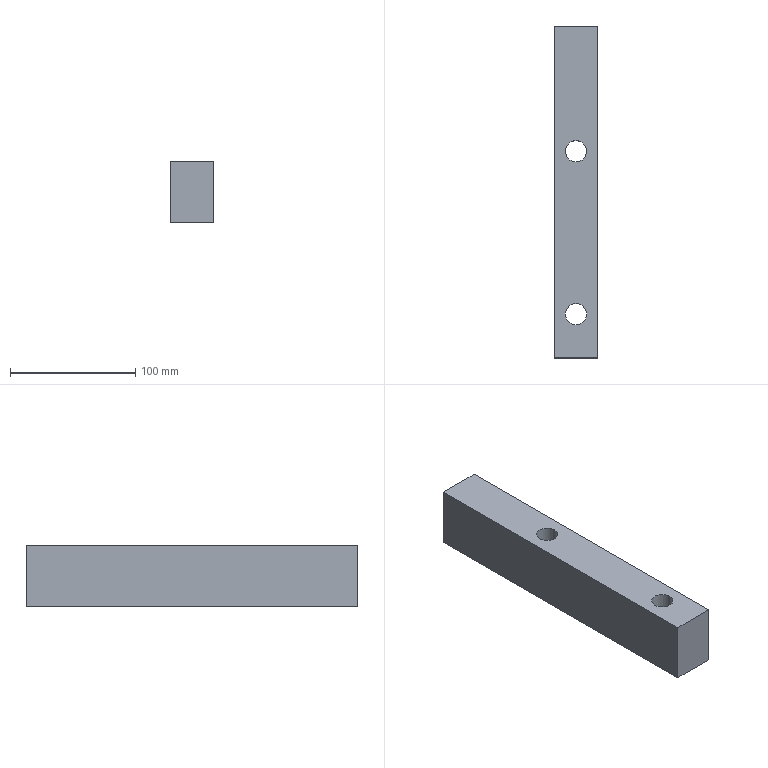Part | NX | features solid 2 | 1 solid | 8 faces | box 35 x 265 x 49 mm | volume 432231 mm3 | plane 6 | cylinder 2 | commonest cylinder face diameters 17 x2
STEP:
#1=CARTESIAN_POINT('',(668.,370.,153.));
#2=VERTEX_POINT('',#1);
#3=CARTESIAN_POINT('',(668.,370.,202.));
#4=VERTEX_POINT('',#3);
#5=CARTESIAN_POINT('',(668.,370.,148.));
#6=DIRECTION('',(0.,0.,1.));
#7=VECTOR('',#6,1000.);
#8=LINE('',#5,#7);
#9=EDGE_CURVE('',#2,#4,#8,.T.);
#10=ORIENTED_EDGE('',*,*,#9,.F.);
#11=CARTESIAN_POINT('',(668.,105.,153.));
#12=VERTEX_POINT('',#11);
#13=CARTESIAN_POINT('',(668.,0.,153.));
#14=DIRECTION('',(0.,-1.,0.));
#15=VECTOR('',#14,1000.);
#16=LINE('',#13,#15);
#17=EDGE_CURVE('',#2,#12,#16,.T.);
#18=ORIENTED_EDGE('',*,*,#17,.T.);
#19=CARTESIAN_POINT('',(668.,105.,202.));
#20=VERTEX_POINT('',#19);
#21=CARTESIAN_POINT('',(668.,105.,148.));
#22=DIRECTION('',(0.,0.,1.));
#23=VECTOR('',#22,1000.);
#24=LINE('',#21,#23);
#25=EDGE_CURVE('',#12,#20,#24,.T.);
#26=ORIENTED_EDGE('',*,*,#25,.T.);
#27=CARTESIAN_POINT('',(668.,0.,202.));
#28=DIRECTION('',(0.,1.,0.));
#29=VECTOR('',#28,1000.);
#30=LINE('',#27,#29);
#31=EDGE_CURVE('',#20,#4,#30,.T.);
#32=ORIENTED_EDGE('',*,*,#31,.T.);
#33=EDGE_LOOP('',(#10,#18,#26,#32));
#34=FACE_BOUND('',#33,.T.);
#35=CARTESIAN_POINT('',(668.,0.,148.));
#36=DIRECTION('',(-1.,0.,0.));
#37=DIRECTION('',(0.,0.,1.));
#38=AXIS2_PLACEMENT_3D('',#35,#36,#37);
#39=PLANE('',#38);
#40=ADVANCED_FACE('',(#34),#39,.T.);
#41=CARTESIAN_POINT('',(703.,370.,153.));
#42=VERTEX_POINT('',#41);
#43=CARTESIAN_POINT('',(703.,370.,202.));
#44=VERTEX_POINT('',#43);
#45=CARTESIAN_POINT('',(703.,370.,148.));
#46=DIRECTION('',(0.,0.,1.));
#47=VECTOR('',#46,1000.);
#48=LINE('',#45,#47);
#49=EDGE_CURVE('',#42,#44,#48,.T.);
#50=ORIENTED_EDGE('',*,*,#49,.F.);
#51=CARTESIAN_POINT('',(685.5,370.,153.));
#52=DIRECTION('',(-1.,0.,0.));
#53=VECTOR('',#52,1000.);
#54=LINE('',#51,#53);
#55=EDGE_CURVE('',#42,#2,#54,.T.);
#56=ORIENTED_EDGE('',*,*,#55,.T.);
#57=ORIENTED_EDGE('',*,*,#9,.T.);
#58=CARTESIAN_POINT('',(685.5,370.,202.));
#59=DIRECTION('',(1.,0.,0.));
#60=VECTOR('',#59,1000.);
#61=LINE('',#58,#60);
#62=EDGE_CURVE('',#4,#44,#61,.T.);
#63=ORIENTED_EDGE('',*,*,#62,.T.);
#64=EDGE_LOOP('',(#50,#56,#57,#63));
#65=FACE_BOUND('',#64,.T.);
#66=CARTESIAN_POINT('',(685.5,370.,148.));
#67=DIRECTION('',(0.,1.,0.));
#68=DIRECTION('',(0.,0.,1.));
#69=AXIS2_PLACEMENT_3D('',#66,#67,#68);
#70=PLANE('',#69);
#71=ADVANCED_FACE('',(#65),#70,.T.);
#72=CARTESIAN_POINT('',(703.,105.,153.));
#73=VERTEX_POINT('',#72);
#74=CARTESIAN_POINT('',(703.,105.,202.));
#75=VERTEX_POINT('',#74);
#76=CARTESIAN_POINT('',(703.,105.,148.));
#77=DIRECTION('',(0.,0.,1.));
#78=VECTOR('',#77,1000.);
#79=LINE('',#76,#78);
#80=EDGE_CURVE('',#73,#75,#79,.T.);
#81=ORIENTED_EDGE('',*,*,#80,.F.);
#82=CARTESIAN_POINT('',(703.,0.,153.));
#83=DIRECTION('',(0.,1.,0.));
#84=VECTOR('',#83,1000.);
#85=LINE('',#82,#84);
#86=EDGE_CURVE('',#73,#42,#85,.T.);
#87=ORIENTED_EDGE('',*,*,#86,.T.);
#88=ORIENTED_EDGE('',*,*,#49,.T.);
#89=CARTESIAN_POINT('',(703.,0.,202.));
#90=DIRECTION('',(0.,-1.,0.));
#91=VECTOR('',#90,1000.);
#92=LINE('',#89,#91);
#93=EDGE_CURVE('',#44,#75,#92,.T.);
#94=ORIENTED_EDGE('',*,*,#93,.T.);
#95=EDGE_LOOP('',(#81,#87,#88,#94));
#96=FACE_BOUND('',#95,.T.);
#97=CARTESIAN_POINT('',(703.,0.,148.));
#98=DIRECTION('',(1.,0.,0.));
#99=DIRECTION('',(0.,0.,-1.));
#100=AXIS2_PLACEMENT_3D('',#97,#98,#99);
#101=PLANE('',#100);
#102=ADVANCED_FACE('',(#96),#101,.T.);
#103=ORIENTED_EDGE('',*,*,#25,.F.);
#104=CARTESIAN_POINT('',(685.5,105.,153.));
#105=DIRECTION('',(1.,0.,0.));
#106=VECTOR('',#105,1000.);
#107=LINE('',#104,#106);
#108=EDGE_CURVE('',#12,#73,#107,.T.);
#109=ORIENTED_EDGE('',*,*,#108,.T.);
#110=ORIENTED_EDGE('',*,*,#80,.T.);
#111=CARTESIAN_POINT('',(685.5,105.,202.));
#112=DIRECTION('',(-1.,0.,0.));
#113=VECTOR('',#112,1000.);
#114=LINE('',#111,#113);
#115=EDGE_CURVE('',#75,#20,#114,.T.);
#116=ORIENTED_EDGE('',*,*,#115,.T.);
#117=EDGE_LOOP('',(#103,#109,#110,#116));
#118=FACE_BOUND('',#117,.T.);
#119=CARTESIAN_POINT('',(685.5,105.,148.));
#120=DIRECTION('',(0.,-1.,0.));
#121=DIRECTION('',(0.,0.,-1.));
#122=AXIS2_PLACEMENT_3D('',#119,#120,#121);
#123=PLANE('',#122);
#124=ADVANCED_FACE('',(#118),#123,.T.);
#125=CARTESIAN_POINT('',(677.,270.,202.));
#126=VERTEX_POINT('',#125);
#127=CARTESIAN_POINT('',(685.5,270.,202.));
#128=DIRECTION('',(0.,0.,-1.));
#129=DIRECTION('',(-1.,0.,0.));
#130=AXIS2_PLACEMENT_3D('',#127,#128,#129);
#131=CIRCLE('',#130,8.5);
#132=EDGE_CURVE('',#126,#126,#131,.T.);
#133=ORIENTED_EDGE('',*,*,#132,.F.);
#134=EDGE_LOOP('',(#133));
#135=FACE_BOUND('',#134,.T.);
#136=CARTESIAN_POINT('',(677.,270.,153.));
#137=VERTEX_POINT('',#136);
#138=CARTESIAN_POINT('',(685.5,270.,153.));
#139=DIRECTION('',(0.,0.,-1.));
#140=DIRECTION('',(-1.,0.,0.));
#141=AXIS2_PLACEMENT_3D('',#138,#139,#140);
#142=CIRCLE('',#141,8.5);
#143=EDGE_CURVE('',#137,#137,#142,.F.);
#144=ORIENTED_EDGE('',*,*,#143,.F.);
#145=EDGE_LOOP('',(#144));
#146=FACE_BOUND('',#145,.T.);
#147=CARTESIAN_POINT('',(685.5,270.,202.));
#148=DIRECTION('',(0.,0.,-1.));
#149=DIRECTION('',(-1.,0.,0.));
#150=AXIS2_PLACEMENT_3D('',#147,#148,#149);
#151=CYLINDRICAL_SURFACE('',#150,8.5);
#152=ADVANCED_FACE('',(#135,#146),#151,.F.);
#153=CARTESIAN_POINT('',(694.,140.,202.));
#154=VERTEX_POINT('',#153);
#155=CARTESIAN_POINT('',(685.5,140.,202.));
#156=DIRECTION('',(0.,0.,1.));
#157=DIRECTION('',(1.,0.,0.));
#158=AXIS2_PLACEMENT_3D('',#155,#156,#157);
#159=CIRCLE('',#158,8.5);
#160=EDGE_CURVE('',#154,#154,#159,.T.);
#161=ORIENTED_EDGE('',*,*,#160,.F.);
#162=EDGE_LOOP('',(#161));
#163=FACE_BOUND('',#162,.T.);
#164=ORIENTED_EDGE('',*,*,#132,.T.);
#165=EDGE_LOOP('',(#164));
#166=FACE_BOUND('',#165,.T.);
#167=ORIENTED_EDGE('',*,*,#115,.F.);
#168=ORIENTED_EDGE('',*,*,#93,.F.);
#169=ORIENTED_EDGE('',*,*,#62,.F.);
#170=ORIENTED_EDGE('',*,*,#31,.F.);
#171=EDGE_LOOP('',(#167,#168,#169,#170));
#172=FACE_BOUND('',#171,.T.);
#173=CARTESIAN_POINT('',(685.5,0.,202.));
#174=DIRECTION('',(0.,0.,1.));
#175=DIRECTION('',(1.,0.,0.));
#176=AXIS2_PLACEMENT_3D('',#173,#174,#175);
#177=PLANE('',#176);
#178=ADVANCED_FACE('',(#163,#166,#172),#177,.T.);
#179=CARTESIAN_POINT('',(677.,140.,153.));
#180=VERTEX_POINT('',#179);
#181=CARTESIAN_POINT('',(685.5,140.,153.));
#182=DIRECTION('',(0.,0.,-1.));
#183=DIRECTION('',(-1.,0.,0.));
#184=AXIS2_PLACEMENT_3D('',#181,#182,#183);
#185=CIRCLE('',#184,8.5);
#186=EDGE_CURVE('',#180,#180,#185,.T.);
#187=ORIENTED_EDGE('',*,*,#186,.F.);
#188=EDGE_LOOP('',(#187));
#189=FACE_BOUND('',#188,.T.);
#190=ORIENTED_EDGE('',*,*,#17,.F.);
#191=ORIENTED_EDGE('',*,*,#55,.F.);
#192=ORIENTED_EDGE('',*,*,#86,.F.);
#193=ORIENTED_EDGE('',*,*,#108,.F.);
#194=EDGE_LOOP('',(#190,#191,#192,#193));
#195=FACE_BOUND('',#194,.T.);
#196=ORIENTED_EDGE('',*,*,#143,.T.);
#197=EDGE_LOOP('',(#196));
#198=FACE_BOUND('',#197,.T.);
#199=CARTESIAN_POINT('',(835.5,0.,153.));
#200=DIRECTION('',(0.,0.,-1.));
#201=DIRECTION('',(-1.,0.,0.));
#202=AXIS2_PLACEMENT_3D('',#199,#200,#201);
#203=PLANE('',#202);
#204=ADVANCED_FACE('',(#189,#195,#198),#203,.T.);
#205=ORIENTED_EDGE('',*,*,#160,.T.);
#206=EDGE_LOOP('',(#205));
#207=FACE_BOUND('',#206,.T.);
#208=ORIENTED_EDGE('',*,*,#186,.T.);
#209=EDGE_LOOP('',(#208));
#210=FACE_BOUND('',#209,.T.);
#211=CARTESIAN_POINT('',(685.5,140.,69.));
#212=DIRECTION('',(0.,0.,1.));
#213=DIRECTION('',(1.,0.,0.));
#214=AXIS2_PLACEMENT_3D('',#211,#212,#213);
#215=CYLINDRICAL_SURFACE('',#214,8.5);
#216=ADVANCED_FACE('',(#207,#210),#215,.F.);
#217=CLOSED_SHELL('',(#40,#71,#102,#124,#152,#178,#204,#216));
#218=MANIFOLD_SOLID_BREP('',#217);
#219=(LENGTH_UNIT()NAMED_UNIT(*)SI_UNIT(.MILLI.,.METRE.));
#220=UNCERTAINTY_MEASURE_WITH_UNIT(LENGTH_MEASURE(0.00001),#219,'','');
#221=(NAMED_UNIT(*)PLANE_ANGLE_UNIT()SI_UNIT($,.RADIAN.));
#222=(NAMED_UNIT(*)SI_UNIT($,.STERADIAN.)SOLID_ANGLE_UNIT());
#223=(GEOMETRIC_REPRESENTATION_CONTEXT(3)GLOBAL_UNCERTAINTY_ASSIGNED_CONTEXT((#220))GLOBAL_UNIT_ASSIGNED_CONTEXT((#219,#221,#222))REPRESENTATION_CONTEXT('',''));
#224=ADVANCED_BREP_SHAPE_REPRESENTATION('',(#218),#223);